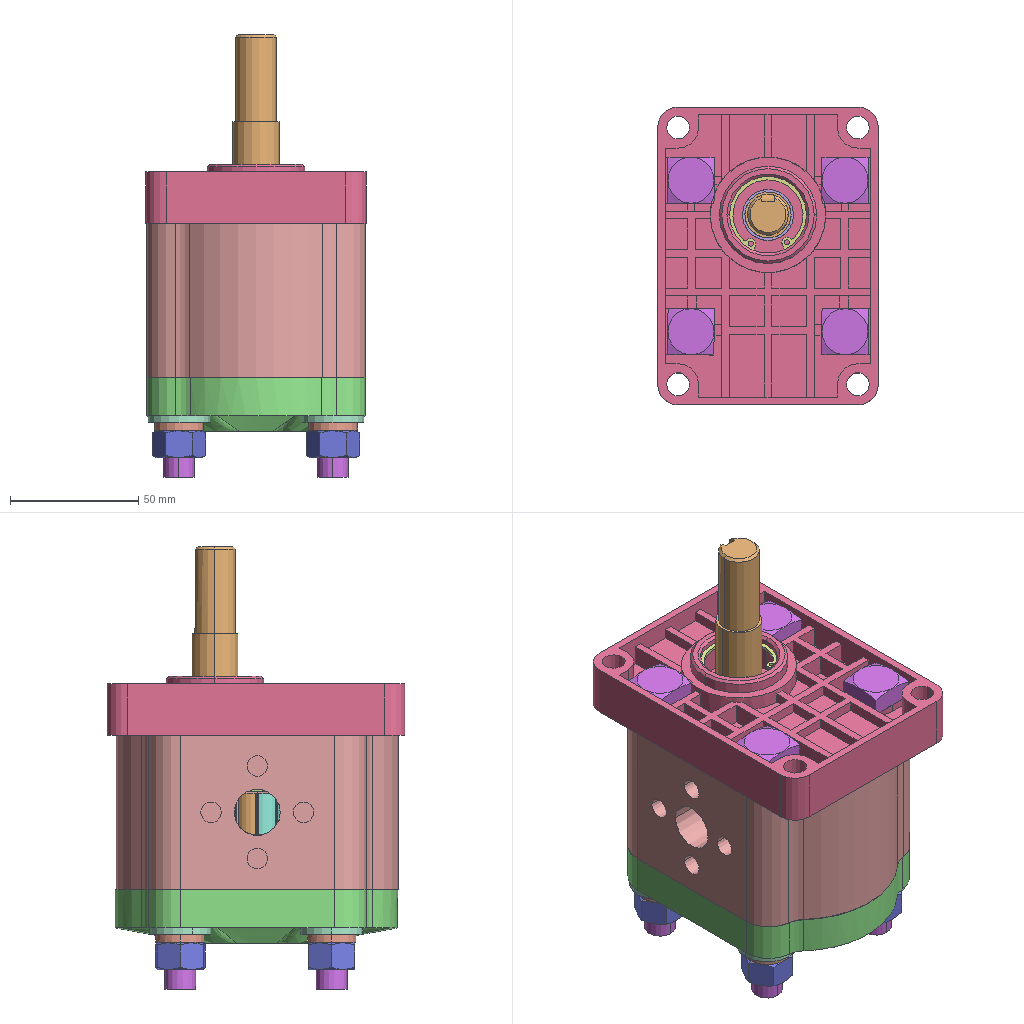Assembly | SolidWorks | 16 different items | 34 placed | box 86 x 116 x 172 mm
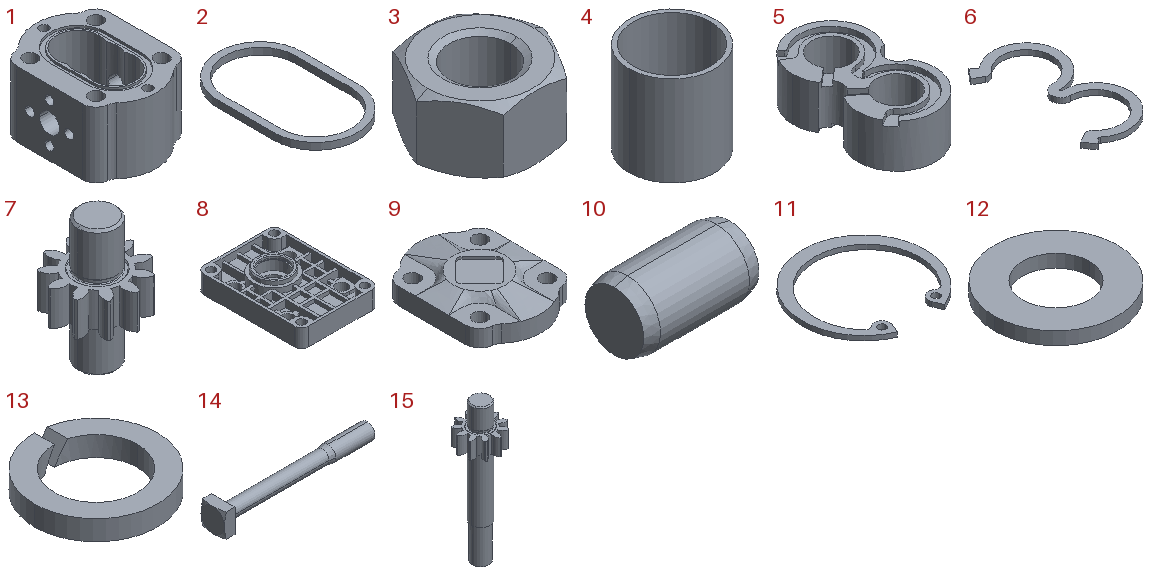Parts list (item | name | quantity | size | volume | features):
1 | - | x1 | 85 x 110 x 60 mm | 289400 mm3 | features ICE 7, MirrorPattern 2, Extrusion 1, Fillet 1
2 | - | x2 | 50 x 83 x 4 mm | 3368 mm3 | features Extrusion 1
3 | - | x4 | 20.785 x 18 x 10.8 mm | 2118 mm3 | features RevCut 2, Chamfer 1, Extrusion 1, LPattern 1
4 | - | x4 | 20 x 20 x 21 mm | 1253 mm3 | features Extrusion 1
5 | - | x2 | 39 x 72 x 22 mm | 33777 mm3 | features ICE 5, Fillet 3, Extrusion 1, MirrorPattern 1
6 | - | x2 | 32.887 x 65 x 2.5 mm | 1343 mm3 | features Fillet 2, Extrusion 1, MirrorPattern 1
7 | - | x1 | 38.724 x 38.336 x 59 mm | 23439 mm3 | features Chamfer 1, Extrusion 1, ICE 1, MirrorPattern 1, RevCut 1
8 | - | x1 | 86 x 116 x 23 mm | 118984 mm3 | features ICE 9, MirrorPattern 2, Chamfer 1, Extrusion 1, RevCut 1
9 | - | x1 | 85 x 110 x 21 mm | 126964 mm3 | features ICE 3, Fillet 2, Blend 1, Extrusion 1
10 | - | x1 | 14 x 8 x 8 mm | 687.093 mm3 | features Revolution 1
11 | - | x1 | 32.1 x 30.878 x 1.2 mm | 259.483 mm3 | features Extrusion 1
12 | - | x4 | 24 x 24 x 2.5 mm | 799.143 mm3 | features Extrusion 1
13 | - | x4 | 19.1 x 19.1 x 3.1 mm | 465.776 mm3 | features Cut 1, Extrusion 1
14 | - | x4 | 118 x 18 x 18 mm | 12442 mm3 | features RevCut 3, Boss 1, Extrusion 1, LPattern 1
15 | - | x1 | 38.724 x 38.336 x 133.5 mm | 40115 mm3 | features ICE 4, Chamfer 1, Extrusion 1, MirrorPattern 1, RevCut 1
16 | parallel pins unhardening steel gb | x1 | - | - | -
Mates (type | each side: item.copy, entity, surface, feature):
Concentric | 1.1 edge | 2.1 edge | 2 times
Coincident | 1.1 face plane Cut-Extrude 3 | 2.1 face plane Boss-Extrude 1
Concentric | 1.1 edge | 2.2 edge | 2 times
Coincident | 1.1 face plane Mirror 1 | 2.2 face plane Boss-Extrude 1
Coincident | 5.1 edge | 6.1 edge
Concentric | 5.2 edge | 6.2 edge | 2 times
Coincident | 5.2 face plane Cut-Extrude 1 | 6.2 face plane Boss-Extrude 1
Concentric | 5.2 edge | 15.1 face cylinder Boss-Extrude 2
Concentric | 5.1 edge | 6.1 edge
Concentric | 7.1 face cylinder Mirror 1 | 4.1 face cylinder Boss-Extrude 1
Concentric | 15.1 face cylinder Boss-Extrude 3 | 4.2 face cylinder Boss-Extrude 1
Concentric | 15.1 face cylinder Boss-Extrude 2 | 4.3 face cylinder Boss-Extrude 1
Concentric | 7.1 face cylinder Boss-Extrude 2 | 4.4 face cylinder Boss-Extrude 1
Coincident | 7.1 face plane Mirror 1 | 4.1 face plane Boss-Extrude 1
Coincident | 15.1 edge | 4.2 edge
Coincident | 15.1 face plane Boss-Extrude 2 | 4.3 face plane Boss-Extrude 1
Coincident | 7.1 face plane Boss-Extrude 2 | 4.4 face plane Boss-Extrude 1
Concentric | 5.2 face cylinder Boss-Extrude 1 | 4.4 face cylinder Boss-Extrude 1
Concentric | 5.1 face cylinder Boss-Extrude 1 | 15.1 face cylinder Boss-Extrude 4
Concentric | 5.1 face cylinder Boss-Extrude 1 | 4.1 face cylinder Boss-Extrude 1
Coincident | 7.1 face plane Boss-Extrude 1 | 15.1 face plane Boss-Extrude 1
Tangent | 7.1 face cylinder Boss-Extrude 1 | 15.1 face cylinder Boss-Extrude 1
Concentric | 1.1 face cylinder Cut-Extrude 2 | 5.2 edge
Concentric | 1.1 face cylinder Cut-Extrude 2 | 5.2 face cylinder Boss-Extrude 1
Coincident | 1.1 face plane Boss-Extrude 1 | 5.2 face plane Boss-Extrude 1
Coincident | 5.2 face plane Boss-Extrude 1 | 15.1 face plane Boss-Extrude 2
Coincident | 1.1 face plane Boss-Extrude 1 | 5.1 face plane Boss-Extrude 1
Concentric | 1.1 face cylinder Cut-Extrude 4 | 8.1 face cylinder Cut-Extrude 4 | 2 times
Concentric | 1.1 face cylinder Cut-Extrude 1 | 9.1 face cylinder Cut-Extrude 2 | 4 times
Coincident | 1.1 face plane Boss-Extrude 1 | 9.1 face plane Boss-Extrude 1
Concentric | 8.1 edge | 11.1 edge
Coincident | 8.1 face plane Cut-Revolve 1 | 11.1 face plane Body
Coincident | 1.1 face plane Boss-Extrude 1 | 8.1 face plane Boss-Extrude 1
Concentric | 1.1 face cylinder Cut-Extrude 1 | 14.1 face cylinder Cut-Revolve1
Concentric | 8.1 face cylinder Cut-Extrude 2 | 14.2 face cylinder Cut-Revolve1
Concentric | 8.1 face cylinder Cut-Extrude 2 | 14.3 face cylinder Cut-Revolve1
Concentric | 8.1 face cylinder Cut-Extrude 2 | 14.4 face cylinder Cut-Revolve1
Coincident | 8.1 face plane Boss-Extrude 6 | 14.1 edge
Coincident | 8.1 face plane Mirror 2 | 14.2 face plane BaseHead
Coincident | 8.1 face plane Boss-Extrude 6 | 14.3 face plane BaseHead
Coincident | 8.1 face plane Mirror 2 | 14.4 face plane BaseHead
Concentric | 14.2 face cylinder BaseBody | 12.1 face cylinder Base-Extrude
Concentric | 14.2 face cylinder BaseBody | 13.1 face cylinder Base-Extrude
Concentric | 14.2 face cylinder BaseBody | 3.1 face cylinder BaseNut
Coincident | 9.1 face plane Boss-Extrude 1 | 12.1 face plane Base-Extrude
Coincident | 12.1 face plane Base-Extrude | 13.1 face plane Base-Extrude
Coincident | 13.1 face plane Base-Extrude | 3.1 face plane BaseNut
Concentric | 14.4 face cylinder BaseBody | 12.2 face cylinder Base-Extrude
Coincident | 9.1 face plane Boss-Extrude 1 | 12.2 face plane Base-Extrude
Concentric | 14.4 face cylinder BaseBody | 13.2 face cylinder Base-Extrude
Coincident | 12.2 face plane Base-Extrude | 13.2 face plane Base-Extrude
Concentric | 14.4 face cylinder BaseBody | 3.2 edge
Coincident | 13.2 face plane Base-Extrude | 3.2 face plane BaseNut
Concentric | 14.1 face cylinder BaseBody | 12.3 face cylinder Base-Extrude
Coincident | 9.1 face plane Boss-Extrude 1 | 12.3 face plane Base-Extrude
Concentric | 14.1 face cylinder BaseBody | 13.3 face cylinder Base-Extrude
Coincident | 12.3 face plane Base-Extrude | 13.3 edge
Concentric | 14.1 face cylinder BaseBody | 3.3 face cylinder BaseNut
Coincident | 13.3 face plane Base-Extrude | 3.3 face plane BaseNut
Concentric | 14.3 face cylinder BaseBody | 12.4 edge
Coincident | 9.1 face plane Boss-Extrude 1 | 12.4 face plane Base-Extrude
Concentric | 14.3 face cylinder BaseBody | 13.4 face cylinder Base-Extrude
Coincident | 12.4 face plane Base-Extrude | 13.4 face plane Base-Extrude
Concentric | 14.3 face cylinder BaseBody | 3.4 face cylinder BaseNut
Coincident | 13.4 face plane Base-Extrude | 3.4 face plane BaseNut